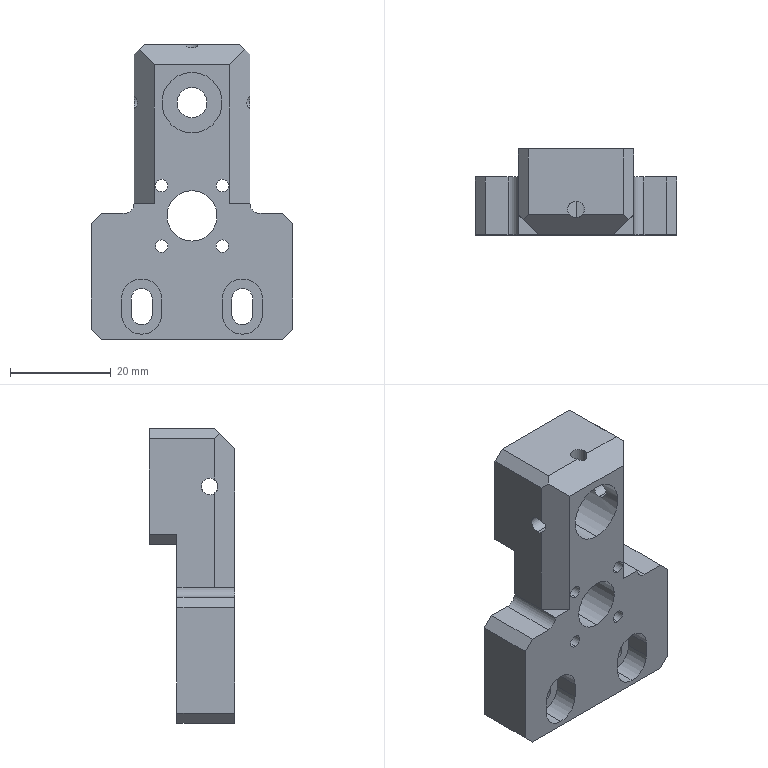Part | SolidWorks | features ICE 9, Chamfer 6, HoleWzd 5, MirrorPattern 3, Fillet 2, MoveFace 2, Extrusion 1 | 1 solid | 89 faces | box 40 x 17 x 58.5 mm | volume 18418 mm3 | cylinder 44 | plane 37 | cone 8 | commonest cylinder face diameters 2.5 x16 3.3 x6 4.2 x6 8 x6 10 x4 4 x2